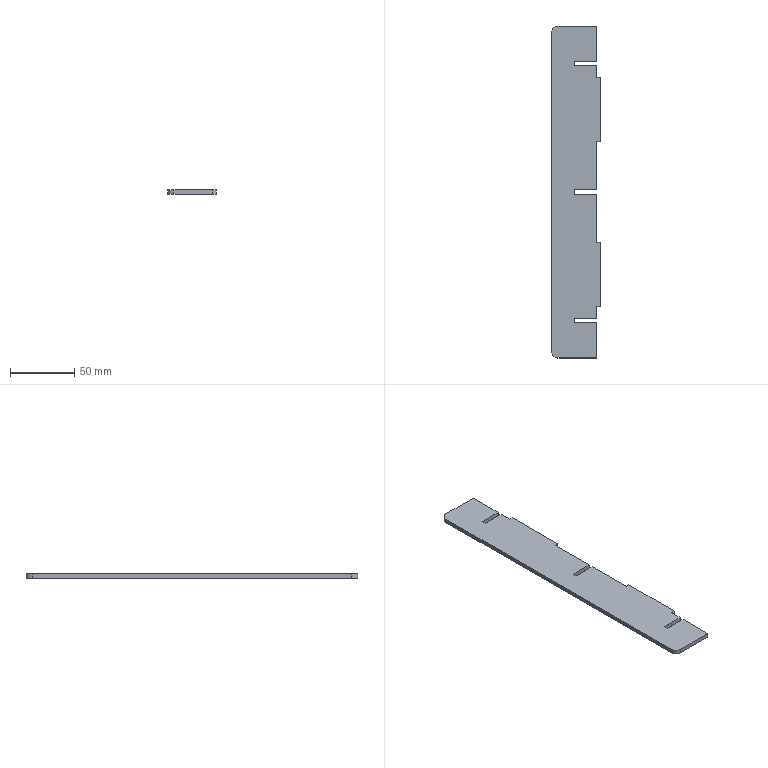Part | SolidWorks | features FlatPattern 1, SMBaseFlange 1, SheetMetal 1 | 1 solid | 28 faces | box 38 x 258 x 3.2 mm | volume 29284 mm3 | plane 26 | cylinder 2 | commonest cylinder face diameters 10 x2
STEP:
#1=CARTESIAN_POINT('',(-320.35,97.96,0.));
#2=VERTEX_POINT('',#1);
#3=CARTESIAN_POINT('',(-320.35,125.36,0.));
#4=VERTEX_POINT('',#3);
#5=CARTESIAN_POINT('',(-320.35,125.36,0.));
#6=DIRECTION('',(0.,1.,0.));
#7=VECTOR('',#6,1000.);
#8=LINE('',#5,#7);
#9=EDGE_CURVE('',#2,#4,#8,.T.);
#10=ORIENTED_EDGE('',*,*,#9,.F.);
#11=CARTESIAN_POINT('',(-320.35,97.96,-3.2));
#12=VERTEX_POINT('',#11);
#13=CARTESIAN_POINT('',(-320.35,97.96,-3.2));
#14=DIRECTION('',(0.,0.,1.));
#15=VECTOR('',#14,1000.);
#16=LINE('',#13,#15);
#17=EDGE_CURVE('',#12,#2,#16,.T.);
#18=ORIENTED_EDGE('',*,*,#17,.F.);
#19=CARTESIAN_POINT('',(-320.35,125.36,-3.2));
#20=VERTEX_POINT('',#19);
#21=CARTESIAN_POINT('',(-320.35,125.36,-3.2));
#22=DIRECTION('',(0.,1.,0.));
#23=VECTOR('',#22,1000.);
#24=LINE('',#21,#23);
#25=EDGE_CURVE('',#12,#20,#24,.T.);
#26=ORIENTED_EDGE('',*,*,#25,.T.);
#27=CARTESIAN_POINT('',(-320.35,125.36,-3.2));
#28=DIRECTION('',(0.,0.,1.));
#29=VECTOR('',#28,1000.);
#30=LINE('',#27,#29);
#31=EDGE_CURVE('',#20,#4,#30,.T.);
#32=ORIENTED_EDGE('',*,*,#31,.T.);
#33=EDGE_LOOP('',(#10,#18,#26,#32));
#34=FACE_OUTER_BOUND('',#33,.T.);
#35=CARTESIAN_POINT('',(-320.35,125.36,-3.2));
#36=DIRECTION('',(1.,0.,0.));
#37=DIRECTION('',(0.,1.,0.));
#38=AXIS2_PLACEMENT_3D('',#35,#36,#37);
#39=PLANE('',#38);
#40=ADVANCED_FACE('',(#34),#39,.T.);
#41=CARTESIAN_POINT('',(-337.85,97.96,0.));
#42=VERTEX_POINT('',#41);
#43=CARTESIAN_POINT('',(-320.35,97.96,0.));
#44=DIRECTION('',(1.,0.,0.));
#45=VECTOR('',#44,1000.);
#46=LINE('',#43,#45);
#47=EDGE_CURVE('',#42,#2,#46,.T.);
#48=ORIENTED_EDGE('',*,*,#47,.F.);
#49=CARTESIAN_POINT('',(-337.85,97.96,-3.2));
#50=VERTEX_POINT('',#49);
#51=CARTESIAN_POINT('',(-337.85,97.96,-3.2));
#52=DIRECTION('',(0.,0.,1.));
#53=VECTOR('',#52,1000.);
#54=LINE('',#51,#53);
#55=EDGE_CURVE('',#50,#42,#54,.T.);
#56=ORIENTED_EDGE('',*,*,#55,.F.);
#57=CARTESIAN_POINT('',(-320.35,97.96,-3.2));
#58=DIRECTION('',(1.,0.,0.));
#59=VECTOR('',#58,1000.);
#60=LINE('',#57,#59);
#61=EDGE_CURVE('',#50,#12,#60,.T.);
#62=ORIENTED_EDGE('',*,*,#61,.T.);
#63=ORIENTED_EDGE('',*,*,#17,.T.);
#64=EDGE_LOOP('',(#48,#56,#62,#63));
#65=FACE_OUTER_BOUND('',#64,.T.);
#66=CARTESIAN_POINT('',(-320.35,97.96,-3.2));
#67=DIRECTION('',(0.,-1.,0.));
#68=DIRECTION('',(0.,0.,-1.));
#69=AXIS2_PLACEMENT_3D('',#66,#67,#68);
#70=PLANE('',#69);
#71=ADVANCED_FACE('',(#65),#70,.T.);
#72=CARTESIAN_POINT('',(-337.85,94.76,0.));
#73=VERTEX_POINT('',#72);
#74=CARTESIAN_POINT('',(-337.85,97.96,0.));
#75=DIRECTION('',(0.,1.,0.));
#76=VECTOR('',#75,1000.);
#77=LINE('',#74,#76);
#78=EDGE_CURVE('',#73,#42,#77,.T.);
#79=ORIENTED_EDGE('',*,*,#78,.F.);
#80=CARTESIAN_POINT('',(-337.85,94.76,-3.2));
#81=VERTEX_POINT('',#80);
#82=CARTESIAN_POINT('',(-337.85,94.76,-3.2));
#83=DIRECTION('',(0.,0.,1.));
#84=VECTOR('',#83,1000.);
#85=LINE('',#82,#84);
#86=EDGE_CURVE('',#81,#73,#85,.T.);
#87=ORIENTED_EDGE('',*,*,#86,.F.);
#88=CARTESIAN_POINT('',(-337.85,97.96,-3.2));
#89=DIRECTION('',(0.,1.,0.));
#90=VECTOR('',#89,1000.);
#91=LINE('',#88,#90);
#92=EDGE_CURVE('',#81,#50,#91,.T.);
#93=ORIENTED_EDGE('',*,*,#92,.T.);
#94=ORIENTED_EDGE('',*,*,#55,.T.);
#95=EDGE_LOOP('',(#79,#87,#93,#94));
#96=FACE_OUTER_BOUND('',#95,.T.);
#97=CARTESIAN_POINT('',(-337.85,97.96,-3.2));
#98=DIRECTION('',(1.,0.,0.));
#99=DIRECTION('',(0.,0.,-1.));
#100=AXIS2_PLACEMENT_3D('',#97,#98,#99);
#101=PLANE('',#100);
#102=ADVANCED_FACE('',(#96),#101,.T.);
#103=CARTESIAN_POINT('',(-320.35,94.76,0.));
#104=VERTEX_POINT('',#103);
#105=CARTESIAN_POINT('',(-337.85,94.76,0.));
#106=DIRECTION('',(-1.,0.,0.));
#107=VECTOR('',#106,1000.);
#108=LINE('',#105,#107);
#109=EDGE_CURVE('',#104,#73,#108,.T.);
#110=ORIENTED_EDGE('',*,*,#109,.F.);
#111=CARTESIAN_POINT('',(-320.35,94.76,-3.2));
#112=VERTEX_POINT('',#111);
#113=CARTESIAN_POINT('',(-320.35,94.76,-3.2));
#114=DIRECTION('',(0.,0.,1.));
#115=VECTOR('',#114,1000.);
#116=LINE('',#113,#115);
#117=EDGE_CURVE('',#112,#104,#116,.T.);
#118=ORIENTED_EDGE('',*,*,#117,.F.);
#119=CARTESIAN_POINT('',(-337.85,94.76,-3.2));
#120=DIRECTION('',(-1.,0.,0.));
#121=VECTOR('',#120,1000.);
#122=LINE('',#119,#121);
#123=EDGE_CURVE('',#112,#81,#122,.T.);
#124=ORIENTED_EDGE('',*,*,#123,.T.);
#125=ORIENTED_EDGE('',*,*,#86,.T.);
#126=EDGE_LOOP('',(#110,#118,#124,#125));
#127=FACE_OUTER_BOUND('',#126,.T.);
#128=CARTESIAN_POINT('',(-337.85,94.76,-3.2));
#129=DIRECTION('',(0.,1.,0.));
#130=DIRECTION('',(0.,0.,1.));
#131=AXIS2_PLACEMENT_3D('',#128,#129,#130);
#132=PLANE('',#131);
#133=ADVANCED_FACE('',(#127),#132,.T.);
#134=CARTESIAN_POINT('',(-320.35,85.36,0.));
#135=VERTEX_POINT('',#134);
#136=CARTESIAN_POINT('',(-320.35,94.76,0.));
#137=DIRECTION('',(0.,1.,0.));
#138=VECTOR('',#137,1000.);
#139=LINE('',#136,#138);
#140=EDGE_CURVE('',#135,#104,#139,.T.);
#141=ORIENTED_EDGE('',*,*,#140,.F.);
#142=CARTESIAN_POINT('',(-320.35,85.36,-3.2));
#143=VERTEX_POINT('',#142);
#144=CARTESIAN_POINT('',(-320.35,85.36,-3.2));
#145=DIRECTION('',(0.,0.,1.));
#146=VECTOR('',#145,1000.);
#147=LINE('',#144,#146);
#148=EDGE_CURVE('',#143,#135,#147,.T.);
#149=ORIENTED_EDGE('',*,*,#148,.F.);
#150=CARTESIAN_POINT('',(-320.35,94.76,-3.2));
#151=DIRECTION('',(0.,1.,0.));
#152=VECTOR('',#151,1000.);
#153=LINE('',#150,#152);
#154=EDGE_CURVE('',#143,#112,#153,.T.);
#155=ORIENTED_EDGE('',*,*,#154,.T.);
#156=ORIENTED_EDGE('',*,*,#117,.T.);
#157=EDGE_LOOP('',(#141,#149,#155,#156));
#158=FACE_OUTER_BOUND('',#157,.T.);
#159=CARTESIAN_POINT('',(-320.35,94.76,-3.2));
#160=DIRECTION('',(1.,0.,0.));
#161=DIRECTION('',(0.,1.,0.));
#162=AXIS2_PLACEMENT_3D('',#159,#160,#161);
#163=PLANE('',#162);
#164=ADVANCED_FACE('',(#158),#163,.T.);
#165=CARTESIAN_POINT('',(-317.35,85.36,0.));
#166=VERTEX_POINT('',#165);
#167=CARTESIAN_POINT('',(-320.35,85.36,0.));
#168=DIRECTION('',(-1.,0.,0.));
#169=VECTOR('',#168,1000.);
#170=LINE('',#167,#169);
#171=EDGE_CURVE('',#166,#135,#170,.T.);
#172=ORIENTED_EDGE('',*,*,#171,.F.);
#173=CARTESIAN_POINT('',(-317.35,85.36,-3.2));
#174=VERTEX_POINT('',#173);
#175=CARTESIAN_POINT('',(-317.35,85.36,-3.2));
#176=DIRECTION('',(0.,0.,1.));
#177=VECTOR('',#176,1000.);
#178=LINE('',#175,#177);
#179=EDGE_CURVE('',#174,#166,#178,.T.);
#180=ORIENTED_EDGE('',*,*,#179,.F.);
#181=CARTESIAN_POINT('',(-320.35,85.36,-3.2));
#182=DIRECTION('',(-1.,0.,0.));
#183=VECTOR('',#182,1000.);
#184=LINE('',#181,#183);
#185=EDGE_CURVE('',#174,#143,#184,.T.);
#186=ORIENTED_EDGE('',*,*,#185,.T.);
#187=ORIENTED_EDGE('',*,*,#148,.T.);
#188=EDGE_LOOP('',(#172,#180,#186,#187));
#189=FACE_OUTER_BOUND('',#188,.T.);
#190=CARTESIAN_POINT('',(-320.35,85.36,-3.2));
#191=DIRECTION('',(0.,1.,0.));
#192=DIRECTION('',(0.,0.,1.));
#193=AXIS2_PLACEMENT_3D('',#190,#191,#192);
#194=PLANE('',#193);
#195=ADVANCED_FACE('',(#189),#194,.T.);
#196=CARTESIAN_POINT('',(-317.35,35.36,0.));
#197=VERTEX_POINT('',#196);
#198=CARTESIAN_POINT('',(-317.35,85.36,0.));
#199=DIRECTION('',(0.,1.,0.));
#200=VECTOR('',#199,1000.);
#201=LINE('',#198,#200);
#202=EDGE_CURVE('',#197,#166,#201,.T.);
#203=ORIENTED_EDGE('',*,*,#202,.F.);
#204=CARTESIAN_POINT('',(-317.35,35.36,-3.2));
#205=VERTEX_POINT('',#204);
#206=CARTESIAN_POINT('',(-317.35,35.36,-3.2));
#207=DIRECTION('',(0.,0.,1.));
#208=VECTOR('',#207,1000.);
#209=LINE('',#206,#208);
#210=EDGE_CURVE('',#205,#197,#209,.T.);
#211=ORIENTED_EDGE('',*,*,#210,.F.);
#212=CARTESIAN_POINT('',(-317.35,85.36,-3.2));
#213=DIRECTION('',(0.,1.,0.));
#214=VECTOR('',#213,1000.);
#215=LINE('',#212,#214);
#216=EDGE_CURVE('',#205,#174,#215,.T.);
#217=ORIENTED_EDGE('',*,*,#216,.T.);
#218=ORIENTED_EDGE('',*,*,#179,.T.);
#219=EDGE_LOOP('',(#203,#211,#217,#218));
#220=FACE_OUTER_BOUND('',#219,.T.);
#221=CARTESIAN_POINT('',(-317.35,85.36,-3.2));
#222=DIRECTION('',(1.,0.,0.));
#223=DIRECTION('',(0.,0.,-1.));
#224=AXIS2_PLACEMENT_3D('',#221,#222,#223);
#225=PLANE('',#224);
#226=ADVANCED_FACE('',(#220),#225,.T.);
#227=CARTESIAN_POINT('',(-320.35,35.36,0.));
#228=VERTEX_POINT('',#227);
#229=CARTESIAN_POINT('',(-317.35,35.36,0.));
#230=DIRECTION('',(1.,0.,0.));
#231=VECTOR('',#230,1000.);
#232=LINE('',#229,#231);
#233=EDGE_CURVE('',#228,#197,#232,.T.);
#234=ORIENTED_EDGE('',*,*,#233,.F.);
#235=CARTESIAN_POINT('',(-320.35,35.36,-3.2));
#236=VERTEX_POINT('',#235);
#237=CARTESIAN_POINT('',(-320.35,35.36,-3.2));
#238=DIRECTION('',(0.,0.,1.));
#239=VECTOR('',#238,1000.);
#240=LINE('',#237,#239);
#241=EDGE_CURVE('',#236,#228,#240,.T.);
#242=ORIENTED_EDGE('',*,*,#241,.F.);
#243=CARTESIAN_POINT('',(-317.35,35.36,-3.2));
#244=DIRECTION('',(1.,0.,0.));
#245=VECTOR('',#244,1000.);
#246=LINE('',#243,#245);
#247=EDGE_CURVE('',#236,#205,#246,.T.);
#248=ORIENTED_EDGE('',*,*,#247,.T.);
#249=ORIENTED_EDGE('',*,*,#210,.T.);
#250=EDGE_LOOP('',(#234,#242,#248,#249));
#251=FACE_OUTER_BOUND('',#250,.T.);
#252=CARTESIAN_POINT('',(-317.35,35.36,-3.2));
#253=DIRECTION('',(0.,-1.,0.));
#254=DIRECTION('',(0.,0.,-1.));
#255=AXIS2_PLACEMENT_3D('',#252,#253,#254);
#256=PLANE('',#255);
#257=ADVANCED_FACE('',(#251),#256,.T.);
#258=CARTESIAN_POINT('',(-320.35,-2.04,0.));
#259=VERTEX_POINT('',#258);
#260=CARTESIAN_POINT('',(-320.35,35.36,0.));
#261=DIRECTION('',(0.,1.,0.));
#262=VECTOR('',#261,1000.);
#263=LINE('',#260,#262);
#264=EDGE_CURVE('',#259,#228,#263,.T.);
#265=ORIENTED_EDGE('',*,*,#264,.F.);
#266=CARTESIAN_POINT('',(-320.35,-2.04,-3.2));
#267=VERTEX_POINT('',#266);
#268=CARTESIAN_POINT('',(-320.35,-2.04,-3.2));
#269=DIRECTION('',(0.,0.,1.));
#270=VECTOR('',#269,1000.);
#271=LINE('',#268,#270);
#272=EDGE_CURVE('',#267,#259,#271,.T.);
#273=ORIENTED_EDGE('',*,*,#272,.F.);
#274=CARTESIAN_POINT('',(-320.35,35.36,-3.2));
#275=DIRECTION('',(0.,1.,0.));
#276=VECTOR('',#275,1000.);
#277=LINE('',#274,#276);
#278=EDGE_CURVE('',#267,#236,#277,.T.);
#279=ORIENTED_EDGE('',*,*,#278,.T.);
#280=ORIENTED_EDGE('',*,*,#241,.T.);
#281=EDGE_LOOP('',(#265,#273,#279,#280));
#282=FACE_OUTER_BOUND('',#281,.T.);
#283=CARTESIAN_POINT('',(-320.35,35.36,-3.2));
#284=DIRECTION('',(1.,0.,0.));
#285=DIRECTION('',(0.,1.,0.));
#286=AXIS2_PLACEMENT_3D('',#283,#284,#285);
#287=PLANE('',#286);
#288=ADVANCED_FACE('',(#282),#287,.T.);
#289=CARTESIAN_POINT('',(-337.85,-2.04,0.));
#290=VERTEX_POINT('',#289);
#291=CARTESIAN_POINT('',(-320.35,-2.04,0.));
#292=DIRECTION('',(1.,0.,0.));
#293=VECTOR('',#292,1000.);
#294=LINE('',#291,#293);
#295=EDGE_CURVE('',#290,#259,#294,.T.);
#296=ORIENTED_EDGE('',*,*,#295,.F.);
#297=CARTESIAN_POINT('',(-337.85,-2.04,-3.2));
#298=VERTEX_POINT('',#297);
#299=CARTESIAN_POINT('',(-337.85,-2.04,-3.2));
#300=DIRECTION('',(0.,0.,1.));
#301=VECTOR('',#300,1000.);
#302=LINE('',#299,#301);
#303=EDGE_CURVE('',#298,#290,#302,.T.);
#304=ORIENTED_EDGE('',*,*,#303,.F.);
#305=CARTESIAN_POINT('',(-320.35,-2.04,-3.2));
#306=DIRECTION('',(1.,0.,0.));
#307=VECTOR('',#306,1000.);
#308=LINE('',#305,#307);
#309=EDGE_CURVE('',#298,#267,#308,.T.);
#310=ORIENTED_EDGE('',*,*,#309,.T.);
#311=ORIENTED_EDGE('',*,*,#272,.T.);
#312=EDGE_LOOP('',(#296,#304,#310,#311));
#313=FACE_OUTER_BOUND('',#312,.T.);
#314=CARTESIAN_POINT('',(-320.35,-2.04,-3.2));
#315=DIRECTION('',(0.,-1.,0.));
#316=DIRECTION('',(0.,0.,-1.));
#317=AXIS2_PLACEMENT_3D('',#314,#315,#316);
#318=PLANE('',#317);
#319=ADVANCED_FACE('',(#313),#318,.T.);
#320=CARTESIAN_POINT('',(-337.85,-5.24,0.));
#321=VERTEX_POINT('',#320);
#322=CARTESIAN_POINT('',(-337.85,-2.04,0.));
#323=DIRECTION('',(0.,1.,0.));
#324=VECTOR('',#323,1000.);
#325=LINE('',#322,#324);
#326=EDGE_CURVE('',#321,#290,#325,.T.);
#327=ORIENTED_EDGE('',*,*,#326,.F.);
#328=CARTESIAN_POINT('',(-337.85,-5.24,-3.2));
#329=VERTEX_POINT('',#328);
#330=CARTESIAN_POINT('',(-337.85,-5.24,-3.2));
#331=DIRECTION('',(0.,0.,1.));
#332=VECTOR('',#331,1000.);
#333=LINE('',#330,#332);
#334=EDGE_CURVE('',#329,#321,#333,.T.);
#335=ORIENTED_EDGE('',*,*,#334,.F.);
#336=CARTESIAN_POINT('',(-337.85,-2.04,-3.2));
#337=DIRECTION('',(0.,1.,0.));
#338=VECTOR('',#337,1000.);
#339=LINE('',#336,#338);
#340=EDGE_CURVE('',#329,#298,#339,.T.);
#341=ORIENTED_EDGE('',*,*,#340,.T.);
#342=ORIENTED_EDGE('',*,*,#303,.T.);
#343=EDGE_LOOP('',(#327,#335,#341,#342));
#344=FACE_OUTER_BOUND('',#343,.T.);
#345=CARTESIAN_POINT('',(-337.85,-2.04,-3.2));
#346=DIRECTION('',(1.,0.,0.));
#347=DIRECTION('',(0.,0.,-1.));
#348=AXIS2_PLACEMENT_3D('',#345,#346,#347);
#349=PLANE('',#348);
#350=ADVANCED_FACE('',(#344),#349,.T.);
#351=CARTESIAN_POINT('',(-320.35,-5.24,0.));
#352=VERTEX_POINT('',#351);
#353=CARTESIAN_POINT('',(-337.85,-5.24,0.));
#354=DIRECTION('',(-1.,0.,0.));
#355=VECTOR('',#354,1000.);
#356=LINE('',#353,#355);
#357=EDGE_CURVE('',#352,#321,#356,.T.);
#358=ORIENTED_EDGE('',*,*,#357,.F.);
#359=CARTESIAN_POINT('',(-320.35,-5.24,-3.2));
#360=VERTEX_POINT('',#359);
#361=CARTESIAN_POINT('',(-320.35,-5.24,-3.2));
#362=DIRECTION('',(0.,0.,1.));
#363=VECTOR('',#362,1000.);
#364=LINE('',#361,#363);
#365=EDGE_CURVE('',#360,#352,#364,.T.);
#366=ORIENTED_EDGE('',*,*,#365,.F.);
#367=CARTESIAN_POINT('',(-337.85,-5.24,-3.2));
#368=DIRECTION('',(-1.,0.,0.));
#369=VECTOR('',#368,1000.);
#370=LINE('',#367,#369);
#371=EDGE_CURVE('',#360,#329,#370,.T.);
#372=ORIENTED_EDGE('',*,*,#371,.T.);
#373=ORIENTED_EDGE('',*,*,#334,.T.);
#374=EDGE_LOOP('',(#358,#366,#372,#373));
#375=FACE_OUTER_BOUND('',#374,.T.);
#376=CARTESIAN_POINT('',(-337.85,-5.24,-3.2));
#377=DIRECTION('',(0.,1.,0.));
#378=DIRECTION('',(0.,0.,1.));
#379=AXIS2_PLACEMENT_3D('',#376,#377,#378);
#380=PLANE('',#379);
#381=ADVANCED_FACE('',(#375),#380,.T.);
#382=CARTESIAN_POINT('',(-320.35,-42.64,0.));
#383=VERTEX_POINT('',#382);
#384=CARTESIAN_POINT('',(-320.35,-5.24,0.));
#385=DIRECTION('',(0.,1.,0.));
#386=VECTOR('',#385,1000.);
#387=LINE('',#384,#386);
#388=EDGE_CURVE('',#383,#352,#387,.T.);
#389=ORIENTED_EDGE('',*,*,#388,.F.);
#390=CARTESIAN_POINT('',(-320.35,-42.64,-3.2));
#391=VERTEX_POINT('',#390);
#392=CARTESIAN_POINT('',(-320.35,-42.64,-3.2));
#393=DIRECTION('',(0.,0.,1.));
#394=VECTOR('',#393,1000.);
#395=LINE('',#392,#394);
#396=EDGE_CURVE('',#391,#383,#395,.T.);
#397=ORIENTED_EDGE('',*,*,#396,.F.);
#398=CARTESIAN_POINT('',(-320.35,-5.24,-3.2));
#399=DIRECTION('',(0.,1.,0.));
#400=VECTOR('',#399,1000.);
#401=LINE('',#398,#400);
#402=EDGE_CURVE('',#391,#360,#401,.T.);
#403=ORIENTED_EDGE('',*,*,#402,.T.);
#404=ORIENTED_EDGE('',*,*,#365,.T.);
#405=EDGE_LOOP('',(#389,#397,#403,#404));
#406=FACE_OUTER_BOUND('',#405,.T.);
#407=CARTESIAN_POINT('',(-320.35,-5.24,-3.2));
#408=DIRECTION('',(1.,0.,0.));
#409=DIRECTION('',(0.,1.,0.));
#410=AXIS2_PLACEMENT_3D('',#407,#408,#409);
#411=PLANE('',#410);
#412=ADVANCED_FACE('',(#406),#411,.T.);
#413=CARTESIAN_POINT('',(-317.35,-42.64,0.));
#414=VERTEX_POINT('',#413);
#415=CARTESIAN_POINT('',(-317.35,-42.64,0.));
#416=DIRECTION('',(-1.,0.,0.));
#417=VECTOR('',#416,1000.);
#418=LINE('',#415,#417);
#419=EDGE_CURVE('',#414,#383,#418,.T.);
#420=ORIENTED_EDGE('',*,*,#419,.F.);
#421=CARTESIAN_POINT('',(-317.35,-42.64,-3.2));
#422=VERTEX_POINT('',#421);
#423=CARTESIAN_POINT('',(-317.35,-42.64,-3.2));
#424=DIRECTION('',(0.,0.,1.));
#425=VECTOR('',#424,1000.);
#426=LINE('',#423,#425);
#427=EDGE_CURVE('',#422,#414,#426,.T.);
#428=ORIENTED_EDGE('',*,*,#427,.F.);
#429=CARTESIAN_POINT('',(-317.35,-42.64,-3.2));
#430=DIRECTION('',(-1.,0.,0.));
#431=VECTOR('',#430,1000.);
#432=LINE('',#429,#431);
#433=EDGE_CURVE('',#422,#391,#432,.T.);
#434=ORIENTED_EDGE('',*,*,#433,.T.);
#435=ORIENTED_EDGE('',*,*,#396,.T.);
#436=EDGE_LOOP('',(#420,#428,#434,#435));
#437=FACE_OUTER_BOUND('',#436,.T.);
#438=CARTESIAN_POINT('',(-317.35,-42.64,-3.2));
#439=DIRECTION('',(0.,1.,0.));
#440=DIRECTION('',(0.,0.,1.));
#441=AXIS2_PLACEMENT_3D('',#438,#439,#440);
#442=PLANE('',#441);
#443=ADVANCED_FACE('',(#437),#442,.T.);
#444=CARTESIAN_POINT('',(-317.35,-92.64,0.));
#445=VERTEX_POINT('',#444);
#446=CARTESIAN_POINT('',(-317.35,-92.64,0.));
#447=DIRECTION('',(0.,1.,0.));
#448=VECTOR('',#447,1000.);
#449=LINE('',#446,#448);
#450=EDGE_CURVE('',#445,#414,#449,.T.);
#451=ORIENTED_EDGE('',*,*,#450,.F.);
#452=CARTESIAN_POINT('',(-317.35,-92.64,-3.2));
#453=VERTEX_POINT('',#452);
#454=CARTESIAN_POINT('',(-317.35,-92.64,-3.2));
#455=DIRECTION('',(0.,0.,1.));
#456=VECTOR('',#455,1000.);
#457=LINE('',#454,#456);
#458=EDGE_CURVE('',#453,#445,#457,.T.);
#459=ORIENTED_EDGE('',*,*,#458,.F.);
#460=CARTESIAN_POINT('',(-317.35,-92.64,-3.2));
#461=DIRECTION('',(0.,1.,0.));
#462=VECTOR('',#461,1000.);
#463=LINE('',#460,#462);
#464=EDGE_CURVE('',#453,#422,#463,.T.);
#465=ORIENTED_EDGE('',*,*,#464,.T.);
#466=ORIENTED_EDGE('',*,*,#427,.T.);
#467=EDGE_LOOP('',(#451,#459,#465,#466));
#468=FACE_OUTER_BOUND('',#467,.T.);
#469=CARTESIAN_POINT('',(-317.35,-92.64,-3.2));
#470=DIRECTION('',(1.,0.,0.));
#471=DIRECTION('',(0.,0.,-1.));
#472=AXIS2_PLACEMENT_3D('',#469,#470,#471);
#473=PLANE('',#472);
#474=ADVANCED_FACE('',(#468),#473,.T.);
#475=CARTESIAN_POINT('',(-320.35,-92.64,0.));
#476=VERTEX_POINT('',#475);
#477=CARTESIAN_POINT('',(-320.35,-92.64,0.));
#478=DIRECTION('',(1.,0.,0.));
#479=VECTOR('',#478,1000.);
#480=LINE('',#477,#479);
#481=EDGE_CURVE('',#476,#445,#480,.T.);
#482=ORIENTED_EDGE('',*,*,#481,.F.);
#483=CARTESIAN_POINT('',(-320.35,-92.64,-3.2));
#484=VERTEX_POINT('',#483);
#485=CARTESIAN_POINT('',(-320.35,-92.64,-3.2));
#486=DIRECTION('',(0.,0.,1.));
#487=VECTOR('',#486,1000.);
#488=LINE('',#485,#487);
#489=EDGE_CURVE('',#484,#476,#488,.T.);
#490=ORIENTED_EDGE('',*,*,#489,.F.);
#491=CARTESIAN_POINT('',(-320.35,-92.64,-3.2));
#492=DIRECTION('',(1.,0.,0.));
#493=VECTOR('',#492,1000.);
#494=LINE('',#491,#493);
#495=EDGE_CURVE('',#484,#453,#494,.T.);
#496=ORIENTED_EDGE('',*,*,#495,.T.);
#497=ORIENTED_EDGE('',*,*,#458,.T.);
#498=EDGE_LOOP('',(#482,#490,#496,#497));
#499=FACE_OUTER_BOUND('',#498,.T.);
#500=CARTESIAN_POINT('',(-320.35,-92.64,-3.2));
#501=DIRECTION('',(0.,-1.,0.));
#502=DIRECTION('',(0.,0.,-1.));
#503=AXIS2_PLACEMENT_3D('',#500,#501,#502);
#504=PLANE('',#503);
#505=ADVANCED_FACE('',(#499),#504,.T.);
#506=CARTESIAN_POINT('',(-320.35,-102.04,0.));
#507=VERTEX_POINT('',#506);
#508=CARTESIAN_POINT('',(-320.35,-92.64,0.));
#509=DIRECTION('',(0.,1.,0.));
#510=VECTOR('',#509,1000.);
#511=LINE('',#508,#510);
#512=EDGE_CURVE('',#507,#476,#511,.T.);
#513=ORIENTED_EDGE('',*,*,#512,.F.);
#514=CARTESIAN_POINT('',(-320.35,-102.04,-3.2));
#515=VERTEX_POINT('',#514);
#516=CARTESIAN_POINT('',(-320.35,-102.04,-3.2));
#517=DIRECTION('',(0.,0.,1.));
#518=VECTOR('',#517,1000.);
#519=LINE('',#516,#518);
#520=EDGE_CURVE('',#515,#507,#519,.T.);
#521=ORIENTED_EDGE('',*,*,#520,.F.);
#522=CARTESIAN_POINT('',(-320.35,-92.64,-3.2));
#523=DIRECTION('',(0.,1.,0.));
#524=VECTOR('',#523,1000.);
#525=LINE('',#522,#524);
#526=EDGE_CURVE('',#515,#484,#525,.T.);
#527=ORIENTED_EDGE('',*,*,#526,.T.);
#528=ORIENTED_EDGE('',*,*,#489,.T.);
#529=EDGE_LOOP('',(#513,#521,#527,#528));
#530=FACE_OUTER_BOUND('',#529,.T.);
#531=CARTESIAN_POINT('',(-320.35,-92.64,-3.2));
#532=DIRECTION('',(1.,0.,0.));
#533=DIRECTION('',(0.,1.,0.));
#534=AXIS2_PLACEMENT_3D('',#531,#532,#533);
#535=PLANE('',#534);
#536=ADVANCED_FACE('',(#530),#535,.T.);
#537=CARTESIAN_POINT('',(-337.85,-102.04,0.));
#538=VERTEX_POINT('',#537);
#539=CARTESIAN_POINT('',(-320.35,-102.04,0.));
#540=DIRECTION('',(1.,0.,0.));
#541=VECTOR('',#540,1000.);
#542=LINE('',#539,#541);
#543=EDGE_CURVE('',#538,#507,#542,.T.);
#544=ORIENTED_EDGE('',*,*,#543,.F.);
#545=CARTESIAN_POINT('',(-337.85,-102.04,-3.2));
#546=VERTEX_POINT('',#545);
#547=CARTESIAN_POINT('',(-337.85,-102.04,-3.2));
#548=DIRECTION('',(0.,0.,1.));
#549=VECTOR('',#548,1000.);
#550=LINE('',#547,#549);
#551=EDGE_CURVE('',#546,#538,#550,.T.);
#552=ORIENTED_EDGE('',*,*,#551,.F.);
#553=CARTESIAN_POINT('',(-320.35,-102.04,-3.2));
#554=DIRECTION('',(1.,0.,0.));
#555=VECTOR('',#554,1000.);
#556=LINE('',#553,#555);
#557=EDGE_CURVE('',#546,#515,#556,.T.);
#558=ORIENTED_EDGE('',*,*,#557,.T.);
#559=ORIENTED_EDGE('',*,*,#520,.T.);
#560=EDGE_LOOP('',(#544,#552,#558,#559));
#561=FACE_OUTER_BOUND('',#560,.T.);
#562=CARTESIAN_POINT('',(-320.35,-102.04,-3.2));
#563=DIRECTION('',(0.,-1.,0.));
#564=DIRECTION('',(0.,0.,-1.));
#565=AXIS2_PLACEMENT_3D('',#562,#563,#564);
#566=PLANE('',#565);
#567=ADVANCED_FACE('',(#561),#566,.T.);
#568=CARTESIAN_POINT('',(-337.85,-105.24,0.));
#569=VERTEX_POINT('',#568);
#570=CARTESIAN_POINT('',(-337.85,-102.04,0.));
#571=DIRECTION('',(0.,1.,0.));
#572=VECTOR('',#571,1000.);
#573=LINE('',#570,#572);
#574=EDGE_CURVE('',#569,#538,#573,.T.);
#575=ORIENTED_EDGE('',*,*,#574,.F.);
#576=CARTESIAN_POINT('',(-337.85,-105.24,-3.2));
#577=VERTEX_POINT('',#576);
#578=CARTESIAN_POINT('',(-337.85,-105.24,-3.2));
#579=DIRECTION('',(0.,0.,1.));
#580=VECTOR('',#579,1000.);
#581=LINE('',#578,#580);
#582=EDGE_CURVE('',#577,#569,#581,.T.);
#583=ORIENTED_EDGE('',*,*,#582,.F.);
#584=CARTESIAN_POINT('',(-337.85,-102.04,-3.2));
#585=DIRECTION('',(0.,1.,0.));
#586=VECTOR('',#585,1000.);
#587=LINE('',#584,#586);
#588=EDGE_CURVE('',#577,#546,#587,.T.);
#589=ORIENTED_EDGE('',*,*,#588,.T.);
#590=ORIENTED_EDGE('',*,*,#551,.T.);
#591=EDGE_LOOP('',(#575,#583,#589,#590));
#592=FACE_OUTER_BOUND('',#591,.T.);
#593=CARTESIAN_POINT('',(-337.85,-102.04,-3.2));
#594=DIRECTION('',(1.,0.,0.));
#595=DIRECTION('',(0.,0.,-1.));
#596=AXIS2_PLACEMENT_3D('',#593,#594,#595);
#597=PLANE('',#596);
#598=ADVANCED_FACE('',(#592),#597,.T.);
#599=CARTESIAN_POINT('',(-320.35,-105.24,0.));
#600=VERTEX_POINT('',#599);
#601=CARTESIAN_POINT('',(-337.85,-105.24,0.));
#602=DIRECTION('',(-1.,0.,0.));
#603=VECTOR('',#602,1000.);
#604=LINE('',#601,#603);
#605=EDGE_CURVE('',#600,#569,#604,.T.);
#606=ORIENTED_EDGE('',*,*,#605,.F.);
#607=CARTESIAN_POINT('',(-320.35,-105.24,-3.2));
#608=VERTEX_POINT('',#607);
#609=CARTESIAN_POINT('',(-320.35,-105.24,-3.2));
#610=DIRECTION('',(0.,0.,1.));
#611=VECTOR('',#610,1000.);
#612=LINE('',#609,#611);
#613=EDGE_CURVE('',#608,#600,#612,.T.);
#614=ORIENTED_EDGE('',*,*,#613,.F.);
#615=CARTESIAN_POINT('',(-337.85,-105.24,-3.2));
#616=DIRECTION('',(-1.,0.,0.));
#617=VECTOR('',#616,1000.);
#618=LINE('',#615,#617);
#619=EDGE_CURVE('',#608,#577,#618,.T.);
#620=ORIENTED_EDGE('',*,*,#619,.T.);
#621=ORIENTED_EDGE('',*,*,#582,.T.);
#622=EDGE_LOOP('',(#606,#614,#620,#621));
#623=FACE_OUTER_BOUND('',#622,.T.);
#624=CARTESIAN_POINT('',(-337.85,-105.24,-3.2));
#625=DIRECTION('',(0.,1.,0.));
#626=DIRECTION('',(0.,0.,1.));
#627=AXIS2_PLACEMENT_3D('',#624,#625,#626);
#628=PLANE('',#627);
#629=ADVANCED_FACE('',(#623),#628,.T.);
#630=CARTESIAN_POINT('',(-320.35,-132.64,0.));
#631=VERTEX_POINT('',#630);
#632=CARTESIAN_POINT('',(-320.35,-105.24,0.));
#633=DIRECTION('',(0.,1.,0.));
#634=VECTOR('',#633,1000.);
#635=LINE('',#632,#634);
#636=EDGE_CURVE('',#631,#600,#635,.T.);
#637=ORIENTED_EDGE('',*,*,#636,.F.);
#638=CARTESIAN_POINT('',(-320.35,-132.64,-3.2));
#639=VERTEX_POINT('',#638);
#640=CARTESIAN_POINT('',(-320.35,-132.64,-3.2));
#641=DIRECTION('',(0.,0.,1.));
#642=VECTOR('',#641,1000.);
#643=LINE('',#640,#642);
#644=EDGE_CURVE('',#639,#631,#643,.T.);
#645=ORIENTED_EDGE('',*,*,#644,.F.);
#646=CARTESIAN_POINT('',(-320.35,-105.24,-3.2));
#647=DIRECTION('',(0.,1.,0.));
#648=VECTOR('',#647,1000.);
#649=LINE('',#646,#648);
#650=EDGE_CURVE('',#639,#608,#649,.T.);
#651=ORIENTED_EDGE('',*,*,#650,.T.);
#652=ORIENTED_EDGE('',*,*,#613,.T.);
#653=EDGE_LOOP('',(#637,#645,#651,#652));
#654=FACE_OUTER_BOUND('',#653,.T.);
#655=CARTESIAN_POINT('',(-320.35,-105.24,-3.2));
#656=DIRECTION('',(1.,0.,0.));
#657=DIRECTION('',(0.,1.,0.));
#658=AXIS2_PLACEMENT_3D('',#655,#656,#657);
#659=PLANE('',#658);
#660=ADVANCED_FACE('',(#654),#659,.T.);
#661=CARTESIAN_POINT('',(-350.35,-132.64,0.));
#662=VERTEX_POINT('',#661);
#663=CARTESIAN_POINT('',(-320.35,-132.64,0.));
#664=DIRECTION('',(1.,0.,0.));
#665=VECTOR('',#664,1000.);
#666=LINE('',#663,#665);
#667=EDGE_CURVE('',#662,#631,#666,.T.);
#668=ORIENTED_EDGE('',*,*,#667,.F.);
#669=CARTESIAN_POINT('',(-350.35,-132.64,-3.2));
#670=VERTEX_POINT('',#669);
#671=CARTESIAN_POINT('',(-350.35,-132.64,-3.2));
#672=DIRECTION('',(0.,0.,1.));
#673=VECTOR('',#672,1000.);
#674=LINE('',#671,#673);
#675=EDGE_CURVE('',#670,#662,#674,.T.);
#676=ORIENTED_EDGE('',*,*,#675,.F.);
#677=CARTESIAN_POINT('',(-320.35,-132.64,-3.2));
#678=DIRECTION('',(1.,0.,0.));
#679=VECTOR('',#678,1000.);
#680=LINE('',#677,#679);
#681=EDGE_CURVE('',#670,#639,#680,.T.);
#682=ORIENTED_EDGE('',*,*,#681,.T.);
#683=ORIENTED_EDGE('',*,*,#644,.T.);
#684=EDGE_LOOP('',(#668,#676,#682,#683));
#685=FACE_OUTER_BOUND('',#684,.T.);
#686=CARTESIAN_POINT('',(-320.35,-132.64,-3.2));
#687=DIRECTION('',(0.,-1.,0.));
#688=DIRECTION('',(0.,0.,-1.));
#689=AXIS2_PLACEMENT_3D('',#686,#687,#688);
#690=PLANE('',#689);
#691=ADVANCED_FACE('',(#685),#690,.T.);
#692=CARTESIAN_POINT('',(-355.35,-127.64,0.));
#693=VERTEX_POINT('',#692);
#694=CARTESIAN_POINT('',(-350.35,-127.64,0.));
#695=DIRECTION('',(0.,0.,1.));
#696=DIRECTION('',(-1.,0.,0.));
#697=AXIS2_PLACEMENT_3D('',#694,#695,#696);
#698=CIRCLE('',#697,5.);
#699=EDGE_CURVE('',#693,#662,#698,.T.);
#700=ORIENTED_EDGE('',*,*,#699,.F.);
#701=CARTESIAN_POINT('',(-355.35,-127.64,-3.2));
#702=VERTEX_POINT('',#701);
#703=CARTESIAN_POINT('',(-355.35,-127.64,-3.2));
#704=DIRECTION('',(0.,0.,1.));
#705=VECTOR('',#704,1000.);
#706=LINE('',#703,#705);
#707=EDGE_CURVE('',#702,#693,#706,.T.);
#708=ORIENTED_EDGE('',*,*,#707,.F.);
#709=CARTESIAN_POINT('',(-350.35,-127.64,-3.2));
#710=DIRECTION('',(0.,0.,1.));
#711=DIRECTION('',(-1.,0.,0.));
#712=AXIS2_PLACEMENT_3D('',#709,#710,#711);
#713=CIRCLE('',#712,5.);
#714=EDGE_CURVE('',#702,#670,#713,.T.);
#715=ORIENTED_EDGE('',*,*,#714,.T.);
#716=ORIENTED_EDGE('',*,*,#675,.T.);
#717=EDGE_LOOP('',(#700,#708,#715,#716));
#718=FACE_OUTER_BOUND('',#717,.T.);
#719=CARTESIAN_POINT('',(-350.35,-127.64,-3.2));
#720=DIRECTION('',(0.,0.,1.));
#721=DIRECTION('',(1.,0.,0.));
#722=AXIS2_PLACEMENT_3D('',#719,#720,#721);
#723=CYLINDRICAL_SURFACE('',#722,5.);
#724=ADVANCED_FACE('',(#718),#723,.T.);
#725=CARTESIAN_POINT('',(-355.35,120.36,0.));
#726=VERTEX_POINT('',#725);
#727=CARTESIAN_POINT('',(-355.35,120.36,0.));
#728=DIRECTION('',(0.,-1.,0.));
#729=VECTOR('',#728,1000.);
#730=LINE('',#727,#729);
#731=EDGE_CURVE('',#726,#693,#730,.T.);
#732=ORIENTED_EDGE('',*,*,#731,.F.);
#733=CARTESIAN_POINT('',(-355.35,120.36,-3.2));
#734=VERTEX_POINT('',#733);
#735=CARTESIAN_POINT('',(-355.35,120.36,-3.2));
#736=DIRECTION('',(0.,0.,1.));
#737=VECTOR('',#736,1000.);
#738=LINE('',#735,#737);
#739=EDGE_CURVE('',#734,#726,#738,.T.);
#740=ORIENTED_EDGE('',*,*,#739,.F.);
#741=CARTESIAN_POINT('',(-355.35,120.36,-3.2));
#742=DIRECTION('',(0.,-1.,0.));
#743=VECTOR('',#742,1000.);
#744=LINE('',#741,#743);
#745=EDGE_CURVE('',#734,#702,#744,.T.);
#746=ORIENTED_EDGE('',*,*,#745,.T.);
#747=ORIENTED_EDGE('',*,*,#707,.T.);
#748=EDGE_LOOP('',(#732,#740,#746,#747));
#749=FACE_OUTER_BOUND('',#748,.T.);
#750=CARTESIAN_POINT('',(-355.35,120.36,-3.2));
#751=DIRECTION('',(-1.,0.,0.));
#752=DIRECTION('',(0.,-1.,0.));
#753=AXIS2_PLACEMENT_3D('',#750,#751,#752);
#754=PLANE('',#753);
#755=ADVANCED_FACE('',(#749),#754,.T.);
#756=CARTESIAN_POINT('',(-350.35,125.36,0.));
#757=VERTEX_POINT('',#756);
#758=CARTESIAN_POINT('',(-350.35,120.36,0.));
#759=DIRECTION('',(0.,0.,1.));
#760=DIRECTION('',(1.,0.,0.));
#761=AXIS2_PLACEMENT_3D('',#758,#759,#760);
#762=CIRCLE('',#761,5.);
#763=EDGE_CURVE('',#757,#726,#762,.T.);
#764=ORIENTED_EDGE('',*,*,#763,.F.);
#765=CARTESIAN_POINT('',(-350.35,125.36,-3.2));
#766=VERTEX_POINT('',#765);
#767=CARTESIAN_POINT('',(-350.35,125.36,-3.2));
#768=DIRECTION('',(0.,0.,1.));
#769=VECTOR('',#768,1000.);
#770=LINE('',#767,#769);
#771=EDGE_CURVE('',#766,#757,#770,.T.);
#772=ORIENTED_EDGE('',*,*,#771,.F.);
#773=CARTESIAN_POINT('',(-350.35,120.36,-3.2));
#774=DIRECTION('',(0.,0.,1.));
#775=DIRECTION('',(1.,0.,0.));
#776=AXIS2_PLACEMENT_3D('',#773,#774,#775);
#777=CIRCLE('',#776,5.);
#778=EDGE_CURVE('',#766,#734,#777,.T.);
#779=ORIENTED_EDGE('',*,*,#778,.T.);
#780=ORIENTED_EDGE('',*,*,#739,.T.);
#781=EDGE_LOOP('',(#764,#772,#779,#780));
#782=FACE_OUTER_BOUND('',#781,.T.);
#783=CARTESIAN_POINT('',(-350.35,120.36,-3.2));
#784=DIRECTION('',(0.,0.,1.));
#785=DIRECTION('',(1.,0.,0.));
#786=AXIS2_PLACEMENT_3D('',#783,#784,#785);
#787=CYLINDRICAL_SURFACE('',#786,5.);
#788=ADVANCED_FACE('',(#782),#787,.T.);
#789=CARTESIAN_POINT('',(-320.35,125.36,0.));
#790=DIRECTION('',(-1.,0.,0.));
#791=VECTOR('',#790,1000.);
#792=LINE('',#789,#791);
#793=EDGE_CURVE('',#4,#757,#792,.T.);
#794=ORIENTED_EDGE('',*,*,#793,.F.);
#795=ORIENTED_EDGE('',*,*,#31,.F.);
#796=CARTESIAN_POINT('',(-320.35,125.36,-3.2));
#797=DIRECTION('',(-1.,0.,0.));
#798=VECTOR('',#797,1000.);
#799=LINE('',#796,#798);
#800=EDGE_CURVE('',#20,#766,#799,.T.);
#801=ORIENTED_EDGE('',*,*,#800,.T.);
#802=ORIENTED_EDGE('',*,*,#771,.T.);
#803=EDGE_LOOP('',(#794,#795,#801,#802));
#804=FACE_OUTER_BOUND('',#803,.T.);
#805=CARTESIAN_POINT('',(-320.35,125.36,-3.2));
#806=DIRECTION('',(0.,1.,0.));
#807=DIRECTION('',(0.,0.,1.));
#808=AXIS2_PLACEMENT_3D('',#805,#806,#807);
#809=PLANE('',#808);
#810=ADVANCED_FACE('',(#804),#809,.T.);
#811=ORIENTED_EDGE('',*,*,#25,.F.);
#812=ORIENTED_EDGE('',*,*,#61,.F.);
#813=ORIENTED_EDGE('',*,*,#92,.F.);
#814=ORIENTED_EDGE('',*,*,#123,.F.);
#815=ORIENTED_EDGE('',*,*,#154,.F.);
#816=ORIENTED_EDGE('',*,*,#185,.F.);
#817=ORIENTED_EDGE('',*,*,#216,.F.);
#818=ORIENTED_EDGE('',*,*,#247,.F.);
#819=ORIENTED_EDGE('',*,*,#278,.F.);
#820=ORIENTED_EDGE('',*,*,#309,.F.);
#821=ORIENTED_EDGE('',*,*,#340,.F.);
#822=ORIENTED_EDGE('',*,*,#371,.F.);
#823=ORIENTED_EDGE('',*,*,#402,.F.);
#824=ORIENTED_EDGE('',*,*,#433,.F.);
#825=ORIENTED_EDGE('',*,*,#464,.F.);
#826=ORIENTED_EDGE('',*,*,#495,.F.);
#827=ORIENTED_EDGE('',*,*,#526,.F.);
#828=ORIENTED_EDGE('',*,*,#557,.F.);
#829=ORIENTED_EDGE('',*,*,#588,.F.);
#830=ORIENTED_EDGE('',*,*,#619,.F.);
#831=ORIENTED_EDGE('',*,*,#650,.F.);
#832=ORIENTED_EDGE('',*,*,#681,.F.);
#833=ORIENTED_EDGE('',*,*,#714,.F.);
#834=ORIENTED_EDGE('',*,*,#745,.F.);
#835=ORIENTED_EDGE('',*,*,#778,.F.);
#836=ORIENTED_EDGE('',*,*,#800,.F.);
#837=EDGE_LOOP('',(#811,#812,#813,#814,#815,#816,#817,#818,#819,#820,#821,#822,#823,#824,#825,#826,#827,#828,#829,#830,#831,#832,#833,#834,#835,#836));
#838=FACE_OUTER_BOUND('',#837,.T.);
#839=CARTESIAN_POINT('',(-350.35,-127.64,-3.2));
#840=DIRECTION('',(0.,0.,-1.));
#841=DIRECTION('',(-1.,0.,0.));
#842=AXIS2_PLACEMENT_3D('',#839,#840,#841);
#843=PLANE('',#842);
#844=ADVANCED_FACE('',(#838),#843,.T.);
#845=ORIENTED_EDGE('',*,*,#9,.T.);
#846=ORIENTED_EDGE('',*,*,#793,.T.);
#847=ORIENTED_EDGE('',*,*,#763,.T.);
#848=ORIENTED_EDGE('',*,*,#731,.T.);
#849=ORIENTED_EDGE('',*,*,#699,.T.);
#850=ORIENTED_EDGE('',*,*,#667,.T.);
#851=ORIENTED_EDGE('',*,*,#636,.T.);
#852=ORIENTED_EDGE('',*,*,#605,.T.);
#853=ORIENTED_EDGE('',*,*,#574,.T.);
#854=ORIENTED_EDGE('',*,*,#543,.T.);
#855=ORIENTED_EDGE('',*,*,#512,.T.);
#856=ORIENTED_EDGE('',*,*,#481,.T.);
#857=ORIENTED_EDGE('',*,*,#450,.T.);
#858=ORIENTED_EDGE('',*,*,#419,.T.);
#859=ORIENTED_EDGE('',*,*,#388,.T.);
#860=ORIENTED_EDGE('',*,*,#357,.T.);
#861=ORIENTED_EDGE('',*,*,#326,.T.);
#862=ORIENTED_EDGE('',*,*,#295,.T.);
#863=ORIENTED_EDGE('',*,*,#264,.T.);
#864=ORIENTED_EDGE('',*,*,#233,.T.);
#865=ORIENTED_EDGE('',*,*,#202,.T.);
#866=ORIENTED_EDGE('',*,*,#171,.T.);
#867=ORIENTED_EDGE('',*,*,#140,.T.);
#868=ORIENTED_EDGE('',*,*,#109,.T.);
#869=ORIENTED_EDGE('',*,*,#78,.T.);
#870=ORIENTED_EDGE('',*,*,#47,.T.);
#871=EDGE_LOOP('',(#845,#846,#847,#848,#849,#850,#851,#852,#853,#854,#855,#856,#857,#858,#859,#860,#861,#862,#863,#864,#865,#866,#867,#868,#869,#870));
#872=FACE_OUTER_BOUND('',#871,.T.);
#873=CARTESIAN_POINT('',(-350.35,-127.64,0.));
#874=DIRECTION('',(0.,0.,-1.));
#875=DIRECTION('',(-1.,0.,0.));
#876=AXIS2_PLACEMENT_3D('',#873,#874,#875);
#877=PLANE('',#876);
#878=ADVANCED_FACE('',(#872),#877,.F.);
#879=CLOSED_SHELL('',(#40,#71,#102,#133,#164,#195,#226,#257,#288,#319,#350,#381,#412,#443,#474,#505,#536,#567,#598,#629,#660,#691,#724,#755,#788,#810,#844,#878));
#880=MANIFOLD_SOLID_BREP('',#879);
#881=CARTESIAN_POINT('',(0.,0.,0.));
#882=DIRECTION('',(0.,0.,1.));
#883=DIRECTION('',(1.,0.,0.));
#884=AXIS2_PLACEMENT_3D('',#881,#882,#883);
#885=(LENGTH_UNIT()NAMED_UNIT(*)SI_UNIT(.MILLI.,.METRE.));
#886=UNCERTAINTY_MEASURE_WITH_UNIT(LENGTH_MEASURE(0.00001),#885,'','');
#887=(NAMED_UNIT(*)PLANE_ANGLE_UNIT()SI_UNIT($,.RADIAN.));
#888=(NAMED_UNIT(*)SI_UNIT($,.STERADIAN.)SOLID_ANGLE_UNIT());
#889=(GEOMETRIC_REPRESENTATION_CONTEXT(3)GLOBAL_UNCERTAINTY_ASSIGNED_CONTEXT((#886))GLOBAL_UNIT_ASSIGNED_CONTEXT((#885,#887,#888))REPRESENTATION_CONTEXT('',''));
#890=ADVANCED_BREP_SHAPE_REPRESENTATION('',(#880,#884),#889);